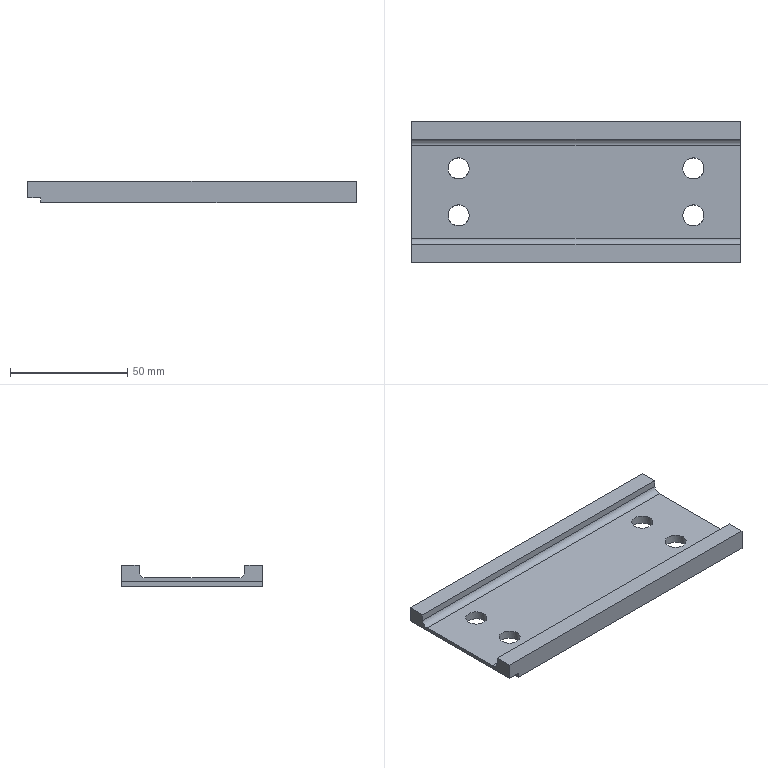Part | STEP file | Tube feed_id22_x_t | 1 solid | 18 faces | box 140 x 60 x 9 mm | volume 40721 mm3 | plane 12 | cylinder 6 | commonest cylinder face diameters 9 x4 5.7 x2